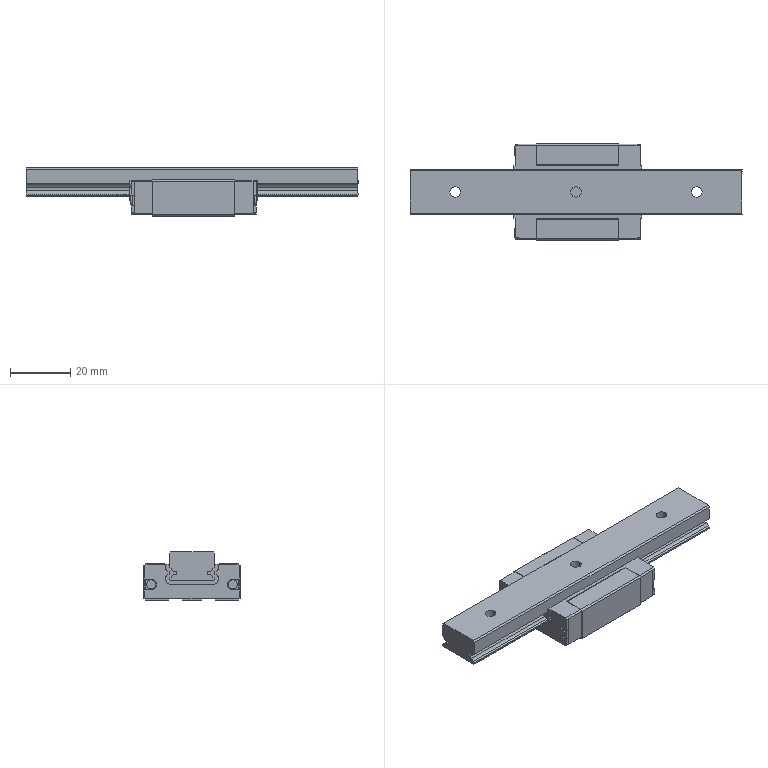Part | SolidWorks | features AEMSimFeature 1 | 2 solids | 305 faces | box 110 x 32 x 16 mm | volume 26387 mm3 | plane 213 | cylinder 76 | cone 16 | commonest cylinder face diameters 3.5 x22 2.459 x8 2.6 x8 3 x8 3.4 x8 0.8 x6